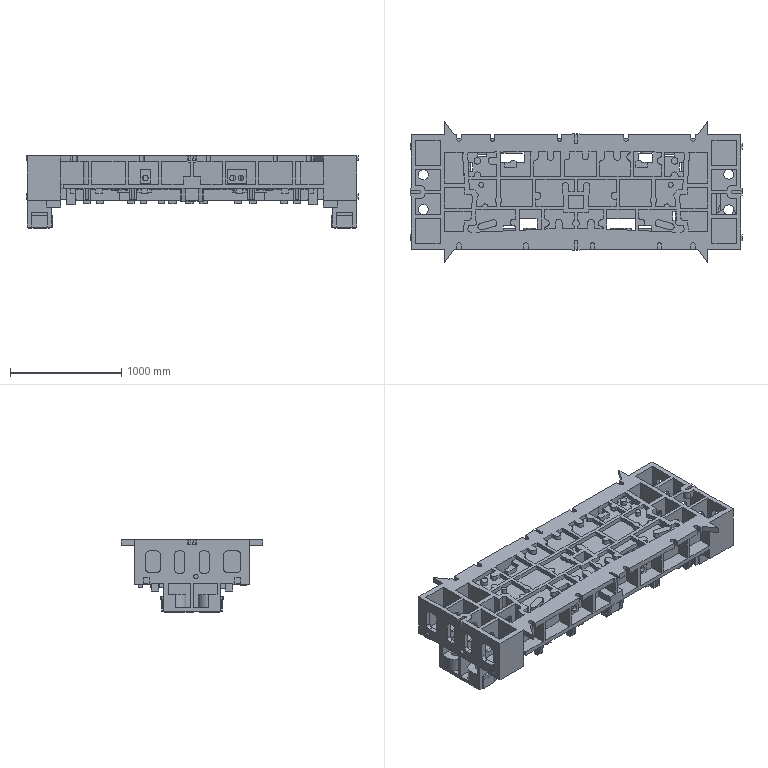Part | NX | features solid 2 | 1 solid | 1881 faces | box 2980 x 1270 x 650 mm | volume 443936836 mm3 | plane 1511 | cylinder 274 | spline 95 | cone 1 | commonest cylinder face diameters 60 x107 40 x34 30 x26 90 x18 120 x12 10 x11